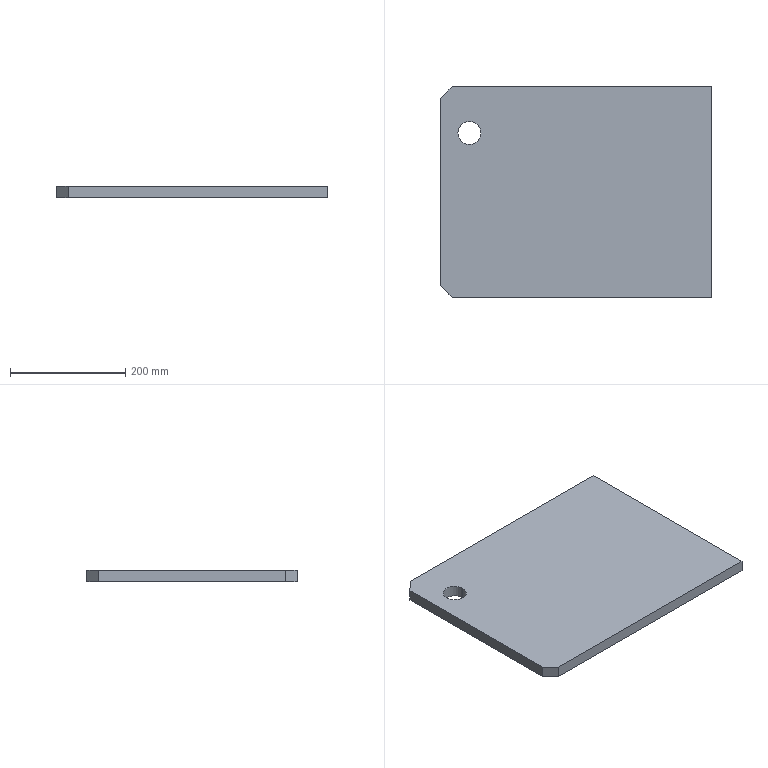Part | SolidWorks | features Chamfer 2, Extrusion 1, ICE 1 | 1 solid | 10 faces | box 470 x 365 x 20 mm | volume 3397867 mm3 | plane 8 | cylinder 2 | commonest cylinder face diameters 40 x2
STEP:
#1=CARTESIAN_POINT('',(-205.,102.5,0.));
#2=VERTEX_POINT('',#1);
#3=CARTESIAN_POINT('',(-165.,102.5,0.));
#4=VERTEX_POINT('',#3);
#5=CARTESIAN_POINT('',(-185.,102.5,0.));
#6=DIRECTION('',(0.,0.,1.));
#7=DIRECTION('',(1.,0.,0.));
#8=AXIS2_PLACEMENT_3D('',#5,#6,#7);
#9=CIRCLE('',#8,20.);
#10=EDGE_CURVE('',#2,#4,#9,.T.);
#11=ORIENTED_EDGE('',*,*,#10,.F.);
#12=CARTESIAN_POINT('',(-205.,102.5,20.));
#13=VERTEX_POINT('',#12);
#14=CARTESIAN_POINT('',(-205.,102.5,0.));
#15=DIRECTION('',(0.,0.,1.));
#16=VECTOR('',#15,1000.);
#17=LINE('',#14,#16);
#18=EDGE_CURVE('',#2,#13,#17,.T.);
#19=ORIENTED_EDGE('',*,*,#18,.T.);
#20=CARTESIAN_POINT('',(-165.,102.5,20.));
#21=VERTEX_POINT('',#20);
#22=CARTESIAN_POINT('',(-185.,102.5,20.));
#23=DIRECTION('',(0.,0.,-1.));
#24=DIRECTION('',(-1.,0.,0.));
#25=AXIS2_PLACEMENT_3D('',#22,#23,#24);
#26=CIRCLE('',#25,20.);
#27=EDGE_CURVE('',#21,#13,#26,.T.);
#28=ORIENTED_EDGE('',*,*,#27,.F.);
#29=CARTESIAN_POINT('',(-165.,102.5,0.));
#30=DIRECTION('',(0.,0.,1.));
#31=VECTOR('',#30,1000.);
#32=LINE('',#29,#31);
#33=EDGE_CURVE('',#4,#21,#32,.T.);
#34=ORIENTED_EDGE('',*,*,#33,.F.);
#35=EDGE_LOOP('',(#11,#19,#28,#34));
#36=FACE_OUTER_BOUND('',#35,.T.);
#37=CARTESIAN_POINT('',(-185.,102.5,0.));
#38=DIRECTION('',(0.,0.,1.));
#39=DIRECTION('',(1.,0.,0.));
#40=AXIS2_PLACEMENT_3D('',#37,#38,#39);
#41=CYLINDRICAL_SURFACE('',#40,20.);
#42=ADVANCED_FACE('',(#36),#41,.F.);
#43=CARTESIAN_POINT('',(-235.,162.5,0.));
#44=VERTEX_POINT('',#43);
#45=CARTESIAN_POINT('',(-235.,-162.5,0.));
#46=VERTEX_POINT('',#45);
#47=CARTESIAN_POINT('',(-235.,182.5,0.));
#48=DIRECTION('',(0.,-1.,0.));
#49=VECTOR('',#48,1000.);
#50=LINE('',#47,#49);
#51=EDGE_CURVE('',#44,#46,#50,.T.);
#52=ORIENTED_EDGE('',*,*,#51,.T.);
#53=CARTESIAN_POINT('',(-235.,-162.5,20.));
#54=VERTEX_POINT('',#53);
#55=CARTESIAN_POINT('',(-235.,-162.5,20.));
#56=DIRECTION('',(0.,0.,1.));
#57=VECTOR('',#56,1000.);
#58=LINE('',#55,#57);
#59=EDGE_CURVE('',#46,#54,#58,.T.);
#60=ORIENTED_EDGE('',*,*,#59,.T.);
#61=CARTESIAN_POINT('',(-235.,162.5,20.));
#62=VERTEX_POINT('',#61);
#63=CARTESIAN_POINT('',(-235.,182.5,20.));
#64=DIRECTION('',(0.,-1.,0.));
#65=VECTOR('',#64,1000.);
#66=LINE('',#63,#65);
#67=EDGE_CURVE('',#62,#54,#66,.T.);
#68=ORIENTED_EDGE('',*,*,#67,.F.);
#69=CARTESIAN_POINT('',(-235.,162.5,20.));
#70=DIRECTION('',(0.,0.,-1.));
#71=VECTOR('',#70,1000.);
#72=LINE('',#69,#71);
#73=EDGE_CURVE('',#62,#44,#72,.T.);
#74=ORIENTED_EDGE('',*,*,#73,.T.);
#75=EDGE_LOOP('',(#52,#60,#68,#74));
#76=FACE_OUTER_BOUND('',#75,.T.);
#77=CARTESIAN_POINT('',(-235.,182.5,20.));
#78=DIRECTION('',(1.,0.,0.));
#79=DIRECTION('',(0.,1.,0.));
#80=AXIS2_PLACEMENT_3D('',#77,#78,#79);
#81=PLANE('',#80);
#82=ADVANCED_FACE('',(#76),#81,.F.);
#83=CARTESIAN_POINT('',(-215.,-182.5,20.));
#84=VERTEX_POINT('',#83);
#85=CARTESIAN_POINT('',(235.,-182.5,20.));
#86=VERTEX_POINT('',#85);
#87=CARTESIAN_POINT('',(235.,-182.5,20.));
#88=DIRECTION('',(1.,0.,0.));
#89=VECTOR('',#88,1000.);
#90=LINE('',#87,#89);
#91=EDGE_CURVE('',#84,#86,#90,.T.);
#92=ORIENTED_EDGE('',*,*,#91,.F.);
#93=CARTESIAN_POINT('',(-215.,-182.5,0.));
#94=VERTEX_POINT('',#93);
#95=CARTESIAN_POINT('',(-215.,-182.5,20.));
#96=DIRECTION('',(0.,0.,-1.));
#97=VECTOR('',#96,1000.);
#98=LINE('',#95,#97);
#99=EDGE_CURVE('',#84,#94,#98,.T.);
#100=ORIENTED_EDGE('',*,*,#99,.T.);
#101=CARTESIAN_POINT('',(235.,-182.5,0.));
#102=VERTEX_POINT('',#101);
#103=CARTESIAN_POINT('',(235.,-182.5,0.));
#104=DIRECTION('',(1.,0.,0.));
#105=VECTOR('',#104,1000.);
#106=LINE('',#103,#105);
#107=EDGE_CURVE('',#94,#102,#106,.T.);
#108=ORIENTED_EDGE('',*,*,#107,.T.);
#109=CARTESIAN_POINT('',(235.,-182.5,20.));
#110=DIRECTION('',(0.,0.,-1.));
#111=VECTOR('',#110,1000.);
#112=LINE('',#109,#111);
#113=EDGE_CURVE('',#86,#102,#112,.T.);
#114=ORIENTED_EDGE('',*,*,#113,.F.);
#115=EDGE_LOOP('',(#92,#100,#108,#114));
#116=FACE_OUTER_BOUND('',#115,.T.);
#117=CARTESIAN_POINT('',(235.,-182.5,20.));
#118=DIRECTION('',(0.,1.,0.));
#119=DIRECTION('',(-1.,0.,0.));
#120=AXIS2_PLACEMENT_3D('',#117,#118,#119);
#121=PLANE('',#120);
#122=ADVANCED_FACE('',(#116),#121,.F.);
#123=CARTESIAN_POINT('',(235.,182.5,0.));
#124=VERTEX_POINT('',#123);
#125=CARTESIAN_POINT('',(235.,182.5,0.));
#126=DIRECTION('',(0.,1.,0.));
#127=VECTOR('',#126,1000.);
#128=LINE('',#125,#127);
#129=EDGE_CURVE('',#102,#124,#128,.T.);
#130=ORIENTED_EDGE('',*,*,#129,.T.);
#131=CARTESIAN_POINT('',(235.,182.5,20.));
#132=VERTEX_POINT('',#131);
#133=CARTESIAN_POINT('',(235.,182.5,20.));
#134=DIRECTION('',(0.,0.,-1.));
#135=VECTOR('',#134,1000.);
#136=LINE('',#133,#135);
#137=EDGE_CURVE('',#132,#124,#136,.T.);
#138=ORIENTED_EDGE('',*,*,#137,.F.);
#139=CARTESIAN_POINT('',(235.,182.5,20.));
#140=DIRECTION('',(0.,1.,0.));
#141=VECTOR('',#140,1000.);
#142=LINE('',#139,#141);
#143=EDGE_CURVE('',#86,#132,#142,.T.);
#144=ORIENTED_EDGE('',*,*,#143,.F.);
#145=ORIENTED_EDGE('',*,*,#113,.T.);
#146=EDGE_LOOP('',(#130,#138,#144,#145));
#147=FACE_OUTER_BOUND('',#146,.T.);
#148=CARTESIAN_POINT('',(235.,182.5,20.));
#149=DIRECTION('',(-1.,0.,0.));
#150=DIRECTION('',(0.,-1.,0.));
#151=AXIS2_PLACEMENT_3D('',#148,#149,#150);
#152=PLANE('',#151);
#153=ADVANCED_FACE('',(#147),#152,.F.);
#154=CARTESIAN_POINT('',(-215.,182.5,0.));
#155=VERTEX_POINT('',#154);
#156=CARTESIAN_POINT('',(235.,182.5,0.));
#157=DIRECTION('',(-1.,0.,0.));
#158=VECTOR('',#157,1000.);
#159=LINE('',#156,#158);
#160=EDGE_CURVE('',#124,#155,#159,.T.);
#161=ORIENTED_EDGE('',*,*,#160,.T.);
#162=CARTESIAN_POINT('',(-215.,182.5,20.));
#163=VERTEX_POINT('',#162);
#164=CARTESIAN_POINT('',(-215.,182.5,20.));
#165=DIRECTION('',(0.,0.,1.));
#166=VECTOR('',#165,1000.);
#167=LINE('',#164,#166);
#168=EDGE_CURVE('',#155,#163,#167,.T.);
#169=ORIENTED_EDGE('',*,*,#168,.T.);
#170=CARTESIAN_POINT('',(235.,182.5,20.));
#171=DIRECTION('',(-1.,0.,0.));
#172=VECTOR('',#171,1000.);
#173=LINE('',#170,#172);
#174=EDGE_CURVE('',#132,#163,#173,.T.);
#175=ORIENTED_EDGE('',*,*,#174,.F.);
#176=ORIENTED_EDGE('',*,*,#137,.T.);
#177=EDGE_LOOP('',(#161,#169,#175,#176));
#178=FACE_OUTER_BOUND('',#177,.T.);
#179=CARTESIAN_POINT('',(235.,182.5,20.));
#180=DIRECTION('',(0.,-1.,0.));
#181=DIRECTION('',(1.,0.,0.));
#182=AXIS2_PLACEMENT_3D('',#179,#180,#181);
#183=PLANE('',#182);
#184=ADVANCED_FACE('',(#178),#183,.F.);
#185=ORIENTED_EDGE('',*,*,#27,.T.);
#186=CARTESIAN_POINT('',(-185.,102.5,20.));
#187=DIRECTION('',(0.,0.,-1.));
#188=DIRECTION('',(-1.,0.,0.));
#189=AXIS2_PLACEMENT_3D('',#186,#187,#188);
#190=CIRCLE('',#189,20.);
#191=EDGE_CURVE('',#13,#21,#190,.T.);
#192=ORIENTED_EDGE('',*,*,#191,.T.);
#193=EDGE_LOOP('',(#185,#192));
#194=FACE_BOUND('',#193,.T.);
#195=ORIENTED_EDGE('',*,*,#67,.T.);
#196=CARTESIAN_POINT('',(-215.,-182.5,20.));
#197=DIRECTION('',(0.7071,-0.7071,0.));
#198=VECTOR('',#197,1000.);
#199=LINE('',#196,#198);
#200=EDGE_CURVE('',#54,#84,#199,.T.);
#201=ORIENTED_EDGE('',*,*,#200,.T.);
#202=ORIENTED_EDGE('',*,*,#91,.T.);
#203=ORIENTED_EDGE('',*,*,#143,.T.);
#204=ORIENTED_EDGE('',*,*,#174,.T.);
#205=CARTESIAN_POINT('',(-235.,162.5,20.));
#206=DIRECTION('',(-0.7071,-0.7071,0.));
#207=VECTOR('',#206,1000.);
#208=LINE('',#205,#207);
#209=EDGE_CURVE('',#163,#62,#208,.T.);
#210=ORIENTED_EDGE('',*,*,#209,.T.);
#211=EDGE_LOOP('',(#195,#201,#202,#203,#204,#210));
#212=FACE_OUTER_BOUND('',#211,.T.);
#213=CARTESIAN_POINT('',(0.,0.,20.));
#214=DIRECTION('',(0.,0.,-1.));
#215=DIRECTION('',(-1.,0.,0.));
#216=AXIS2_PLACEMENT_3D('',#213,#214,#215);
#217=PLANE('',#216);
#218=ADVANCED_FACE('',(#194,#212),#217,.F.);
#219=CARTESIAN_POINT('',(-185.,102.5,0.));
#220=DIRECTION('',(0.,0.,1.));
#221=DIRECTION('',(1.,0.,0.));
#222=AXIS2_PLACEMENT_3D('',#219,#220,#221);
#223=CIRCLE('',#222,20.);
#224=EDGE_CURVE('',#4,#2,#223,.T.);
#225=ORIENTED_EDGE('',*,*,#224,.T.);
#226=ORIENTED_EDGE('',*,*,#10,.T.);
#227=EDGE_LOOP('',(#225,#226));
#228=FACE_BOUND('',#227,.T.);
#229=ORIENTED_EDGE('',*,*,#107,.F.);
#230=CARTESIAN_POINT('',(-198.75,-198.75,0.));
#231=DIRECTION('',(-0.7071,0.7071,0.));
#232=VECTOR('',#231,1000.);
#233=LINE('',#230,#232);
#234=EDGE_CURVE('',#94,#46,#233,.T.);
#235=ORIENTED_EDGE('',*,*,#234,.T.);
#236=ORIENTED_EDGE('',*,*,#51,.F.);
#237=CARTESIAN_POINT('',(-198.75,198.75,0.));
#238=DIRECTION('',(0.7071,0.7071,0.));
#239=VECTOR('',#238,1000.);
#240=LINE('',#237,#239);
#241=EDGE_CURVE('',#44,#155,#240,.T.);
#242=ORIENTED_EDGE('',*,*,#241,.T.);
#243=ORIENTED_EDGE('',*,*,#160,.F.);
#244=ORIENTED_EDGE('',*,*,#129,.F.);
#245=EDGE_LOOP('',(#229,#235,#236,#242,#243,#244));
#246=FACE_OUTER_BOUND('',#245,.T.);
#247=CARTESIAN_POINT('',(0.,0.,0.));
#248=DIRECTION('',(0.,0.,-1.));
#249=DIRECTION('',(-1.,0.,0.));
#250=AXIS2_PLACEMENT_3D('',#247,#248,#249);
#251=PLANE('',#250);
#252=ADVANCED_FACE('',(#228,#246),#251,.T.);
#253=ORIENTED_EDGE('',*,*,#209,.F.);
#254=ORIENTED_EDGE('',*,*,#168,.F.);
#255=ORIENTED_EDGE('',*,*,#241,.F.);
#256=ORIENTED_EDGE('',*,*,#73,.F.);
#257=EDGE_LOOP('',(#253,#254,#255,#256));
#258=FACE_OUTER_BOUND('',#257,.T.);
#259=CARTESIAN_POINT('',(-235.,162.5,20.));
#260=DIRECTION('',(0.7071,-0.7071,0.));
#261=DIRECTION('',(0.,0.,-1.));
#262=AXIS2_PLACEMENT_3D('',#259,#260,#261);
#263=PLANE('',#262);
#264=ADVANCED_FACE('',(#258),#263,.F.);
#265=ORIENTED_EDGE('',*,*,#18,.F.);
#266=ORIENTED_EDGE('',*,*,#224,.F.);
#267=ORIENTED_EDGE('',*,*,#33,.T.);
#268=ORIENTED_EDGE('',*,*,#191,.F.);
#269=EDGE_LOOP('',(#265,#266,#267,#268));
#270=FACE_OUTER_BOUND('',#269,.T.);
#271=CARTESIAN_POINT('',(-185.,102.5,0.));
#272=DIRECTION('',(0.,0.,1.));
#273=DIRECTION('',(1.,0.,0.));
#274=AXIS2_PLACEMENT_3D('',#271,#272,#273);
#275=CYLINDRICAL_SURFACE('',#274,20.);
#276=ADVANCED_FACE('',(#270),#275,.F.);
#277=ORIENTED_EDGE('',*,*,#200,.F.);
#278=ORIENTED_EDGE('',*,*,#59,.F.);
#279=ORIENTED_EDGE('',*,*,#234,.F.);
#280=ORIENTED_EDGE('',*,*,#99,.F.);
#281=EDGE_LOOP('',(#277,#278,#279,#280));
#282=FACE_OUTER_BOUND('',#281,.T.);
#283=CARTESIAN_POINT('',(-215.,-182.5,20.));
#284=DIRECTION('',(0.7071,0.7071,0.));
#285=DIRECTION('',(0.,0.,-1.));
#286=AXIS2_PLACEMENT_3D('',#283,#284,#285);
#287=PLANE('',#286);
#288=ADVANCED_FACE('',(#282),#287,.F.);
#289=CLOSED_SHELL('',(#42,#82,#122,#153,#184,#218,#252,#264,#276,#288));
#290=MANIFOLD_SOLID_BREP('',#289);
#291=CARTESIAN_POINT('',(0.,0.,0.));
#292=DIRECTION('',(0.,0.,1.));
#293=DIRECTION('',(1.,0.,0.));
#294=AXIS2_PLACEMENT_3D('',#291,#292,#293);
#295=(LENGTH_UNIT()NAMED_UNIT(*)SI_UNIT(.MILLI.,.METRE.));
#296=UNCERTAINTY_MEASURE_WITH_UNIT(LENGTH_MEASURE(0.00001),#295,'','');
#297=(NAMED_UNIT(*)PLANE_ANGLE_UNIT()SI_UNIT($,.RADIAN.));
#298=(NAMED_UNIT(*)SI_UNIT($,.STERADIAN.)SOLID_ANGLE_UNIT());
#299=(GEOMETRIC_REPRESENTATION_CONTEXT(3)GLOBAL_UNCERTAINTY_ASSIGNED_CONTEXT((#296))GLOBAL_UNIT_ASSIGNED_CONTEXT((#295,#297,#298))REPRESENTATION_CONTEXT('',''));
#300=ADVANCED_BREP_SHAPE_REPRESENTATION('',(#290,#294),#299);